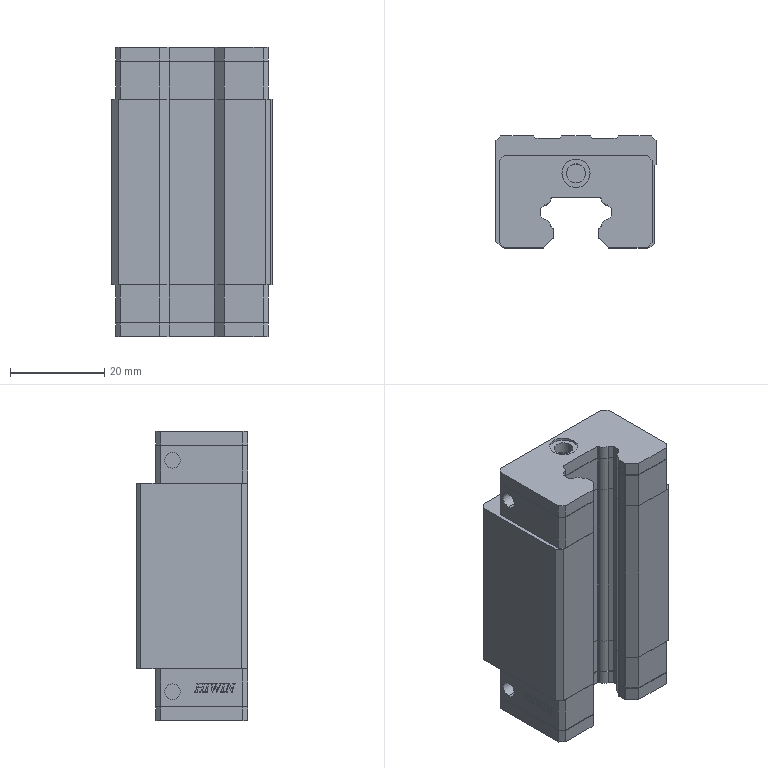Part | STEP file | 5 solids | 606 faces | box 34 x 23.7 x 61.4 mm | volume 36598 mm3 | plane 478 | cylinder 96 | cone 32 | commonest cylinder face diameters 0.8 x40 3.24 x20 3.242 x8 3.3 x8 4 x8 1 x4